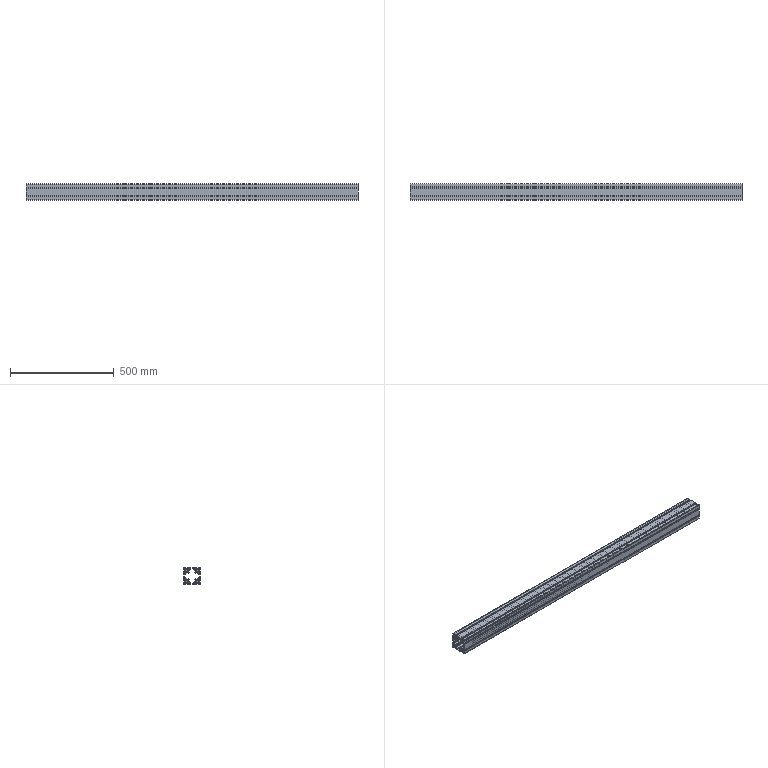Part | SolidWorks | features ICE 1, WeldMemberFeat 1, WeldmentFeature 1 | 1 solid | 174 faces | box 1600 x 80 x 80 mm | volume 3662433 mm3 | plane 146 | cylinder 28 | commonest cylinder face diameters 2 x8 6 x8 6.8 x8 3 x4